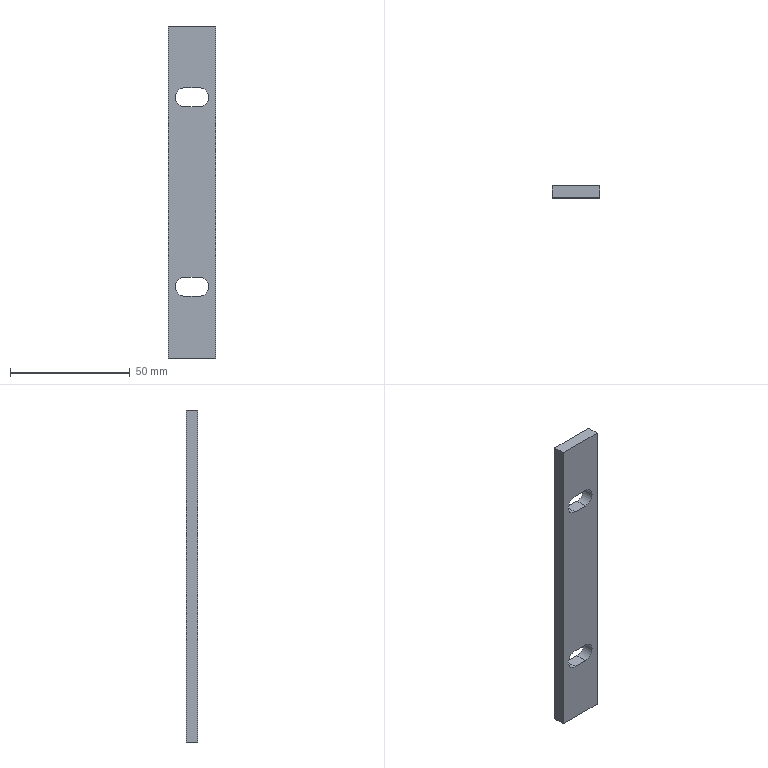Part | STEP file | PRT0001_68_17 | 1 solid | 14 faces | box 20 x 5 x 138.552 mm | volume 12873 mm3 | plane 10 | cylinder 4 | commonest cylinder face diameters 8 x4
STEP:
#1=CARTESIAN_POINT('',(0.,0.,0.));
#2=DIRECTION('',(0.,0.,1.));
#3=DIRECTION('',(1.,0.,0.));
#4=AXIS2_PLACEMENT_3D('',#1,#2,#3);
#5=CARTESIAN_POINT('',(1371.462,1237.457,35.5));
#6=VERTEX_POINT('',#5);
#7=CARTESIAN_POINT('',(1377.462,1237.457,35.5));
#8=VERTEX_POINT('',#7);
#9=CARTESIAN_POINT('',(1371.462,1237.457,35.5));
#10=DIRECTION('',(1.,0.,0.));
#11=VECTOR('',#10,1.);
#12=LINE('',#9,#11);
#13=CARTESIAN_POINT('',(1377.462,1242.457,35.5));
#14=DIRECTION('',(0.,0.,-1.));
#15=DIRECTION('',(-1.,0.,0.));
#16=AXIS2_PLACEMENT_3D('',#13,#14,#15);
#17=PLANE('',#16);
#18=CARTESIAN_POINT('',(6.,-5.));
#19=DIRECTION('',(-1.,0.));
#20=VECTOR('',#19,1.);
#21=LINE('',#18,#20);
#22=(GEOMETRIC_REPRESENTATION_CONTEXT(2)PARAMETRIC_REPRESENTATION_CONTEXT()REPRESENTATION_CONTEXT('',''));
#23=DEFINITIONAL_REPRESENTATION('',(#21),#22);
#24=PCURVE('',#17,#23);
#25=CARTESIAN_POINT('',(1364.462,1237.457,72.014));
#26=DIRECTION('',(0.,-1.,0.));
#27=DIRECTION('',(1.,0.,0.));
#28=AXIS2_PLACEMENT_3D('',#25,#26,#27);
#29=PLANE('',#28);
#30=CARTESIAN_POINT('',(7.,-36.514));
#31=DIRECTION('',(1.,0.));
#32=VECTOR('',#31,1.);
#33=LINE('',#30,#32);
#34=(GEOMETRIC_REPRESENTATION_CONTEXT(2)PARAMETRIC_REPRESENTATION_CONTEXT()REPRESENTATION_CONTEXT('',''));
#35=DEFINITIONAL_REPRESENTATION('',(#33),#34);
#36=PCURVE('',#29,#35);
#37=SURFACE_CURVE('',#12,(#24,#36),.PCURVE_S1.);
#38=EDGE_CURVE('',#6,#8,#37,.T.);
#39=ORIENTED_EDGE('',*,*,#38,.F.);
#40=CARTESIAN_POINT('',(1371.462,1242.457,35.5));
#41=VERTEX_POINT('',#40);
#42=CARTESIAN_POINT('',(1371.462,1242.457,35.5));
#43=DIRECTION('',(0.,-1.,0.));
#44=VECTOR('',#43,1.);
#45=LINE('',#42,#44);
#46=CARTESIAN_POINT('',(6.,0.00006163));
#47=DIRECTION('',(0.,-1.));
#48=VECTOR('',#47,1.);
#49=LINE('',#46,#48);
#50=(GEOMETRIC_REPRESENTATION_CONTEXT(2)PARAMETRIC_REPRESENTATION_CONTEXT()REPRESENTATION_CONTEXT('',''));
#51=DEFINITIONAL_REPRESENTATION('',(#49),#50);
#52=PCURVE('',#17,#51);
#53=CARTESIAN_POINT('',(1371.462,1242.457,39.5));
#54=DIRECTION('',(0.,1.,0.));
#55=DIRECTION('',(1.,0.,0.));
#56=AXIS2_PLACEMENT_3D('',#53,#54,#55);
#57=CYLINDRICAL_SURFACE('',#56,4.);
#58=CARTESIAN_POINT('',(1.571,0.00006163));
#59=DIRECTION('',(0.,-1.));
#60=VECTOR('',#59,1.);
#61=LINE('',#58,#60);
#62=(GEOMETRIC_REPRESENTATION_CONTEXT(2)PARAMETRIC_REPRESENTATION_CONTEXT()REPRESENTATION_CONTEXT('',''));
#63=DEFINITIONAL_REPRESENTATION('',(#61),#62);
#64=PCURVE('',#57,#63);
#65=SURFACE_CURVE('',#45,(#52,#64),.PCURVE_S1.);
#66=EDGE_CURVE('',#41,#6,#65,.T.);
#67=ORIENTED_EDGE('',*,*,#66,.F.);
#68=CARTESIAN_POINT('',(1377.462,1242.457,35.5));
#69=VERTEX_POINT('',#68);
#70=CARTESIAN_POINT('',(1371.462,1242.457,35.5));
#71=DIRECTION('',(1.,0.,0.));
#72=VECTOR('',#71,1.);
#73=LINE('',#70,#72);
#74=CARTESIAN_POINT('',(6.,0.00006163));
#75=DIRECTION('',(-1.,0.));
#76=VECTOR('',#75,1.);
#77=LINE('',#74,#76);
#78=(GEOMETRIC_REPRESENTATION_CONTEXT(2)PARAMETRIC_REPRESENTATION_CONTEXT()REPRESENTATION_CONTEXT('',''));
#79=DEFINITIONAL_REPRESENTATION('',(#77),#78);
#80=PCURVE('',#17,#79);
#81=CARTESIAN_POINT('',(1384.462,1242.457,72.014));
#82=DIRECTION('',(0.,1.,0.));
#83=DIRECTION('',(-1.,0.,0.));
#84=AXIS2_PLACEMENT_3D('',#81,#82,#83);
#85=PLANE('',#84);
#86=CARTESIAN_POINT('',(13.,-36.514));
#87=DIRECTION('',(-1.,0.));
#88=VECTOR('',#87,1.);
#89=LINE('',#86,#88);
#90=(GEOMETRIC_REPRESENTATION_CONTEXT(2)PARAMETRIC_REPRESENTATION_CONTEXT()REPRESENTATION_CONTEXT('',''));
#91=DEFINITIONAL_REPRESENTATION('',(#89),#90);
#92=PCURVE('',#85,#91);
#93=SURFACE_CURVE('',#73,(#80,#92),.PCURVE_S1.);
#94=EDGE_CURVE('',#41,#69,#93,.T.);
#95=ORIENTED_EDGE('',*,*,#94,.T.);
#96=CARTESIAN_POINT('',(1377.462,1237.457,35.5));
#97=DIRECTION('',(0.,1.,0.));
#98=VECTOR('',#97,1.);
#99=LINE('',#96,#98);
#100=CARTESIAN_POINT('',(0.,-5.));
#101=DIRECTION('',(0.,1.));
#102=VECTOR('',#101,1.);
#103=LINE('',#100,#102);
#104=(GEOMETRIC_REPRESENTATION_CONTEXT(2)PARAMETRIC_REPRESENTATION_CONTEXT()REPRESENTATION_CONTEXT('',''));
#105=DEFINITIONAL_REPRESENTATION('',(#103),#104);
#106=PCURVE('',#17,#105);
#107=CARTESIAN_POINT('',(1377.462,1242.457,39.5));
#108=DIRECTION('',(0.,1.,0.));
#109=DIRECTION('',(1.,0.,0.));
#110=AXIS2_PLACEMENT_3D('',#107,#108,#109);
#111=CYLINDRICAL_SURFACE('',#110,4.);
#112=CARTESIAN_POINT('',(1.571,-5.));
#113=DIRECTION('',(0.,1.));
#114=VECTOR('',#113,1.);
#115=LINE('',#112,#114);
#116=(GEOMETRIC_REPRESENTATION_CONTEXT(2)PARAMETRIC_REPRESENTATION_CONTEXT()REPRESENTATION_CONTEXT('',''));
#117=DEFINITIONAL_REPRESENTATION('',(#115),#116);
#118=PCURVE('',#111,#117);
#119=SURFACE_CURVE('',#99,(#106,#118),.PCURVE_S1.);
#120=EDGE_CURVE('',#8,#69,#119,.T.);
#121=ORIENTED_EDGE('',*,*,#120,.F.);
#122=EDGE_LOOP('',(#39,#67,#95,#121));
#123=FACE_BOUND('',#122,.F.);
#124=ADVANCED_FACE('',(#123),#17,.F.);
#125=CARTESIAN_POINT('',(1384.462,1237.457,-69.276));
#126=VERTEX_POINT('',#125);
#127=CARTESIAN_POINT('',(1364.462,1237.457,-69.276));
#128=VERTEX_POINT('',#127);
#129=CARTESIAN_POINT('',(1384.462,1237.457,-69.276));
#130=DIRECTION('',(-1.,0.,0.));
#131=VECTOR('',#130,1.);
#132=LINE('',#129,#131);
#133=CARTESIAN_POINT('',(20.,-141.29));
#134=DIRECTION('',(-1.,0.));
#135=VECTOR('',#134,1.);
#136=LINE('',#133,#135);
#137=(GEOMETRIC_REPRESENTATION_CONTEXT(2)PARAMETRIC_REPRESENTATION_CONTEXT()REPRESENTATION_CONTEXT('',''));
#138=DEFINITIONAL_REPRESENTATION('',(#136),#137);
#139=PCURVE('',#29,#138);
#140=CARTESIAN_POINT('',(1605.102,1107.827,-69.276));
#141=DIRECTION('',(0.,0.,-1.));
#142=DIRECTION('',(-1.,0.,0.));
#143=AXIS2_PLACEMENT_3D('',#140,#141,#142);
#144=PLANE('',#143);
#145=CARTESIAN_POINT('',(220.639,129.63));
#146=DIRECTION('',(1.,0.));
#147=VECTOR('',#146,1.);
#148=LINE('',#145,#147);
#149=(GEOMETRIC_REPRESENTATION_CONTEXT(2)PARAMETRIC_REPRESENTATION_CONTEXT()REPRESENTATION_CONTEXT('',''));
#150=DEFINITIONAL_REPRESENTATION('',(#148),#149);
#151=PCURVE('',#144,#150);
#152=SURFACE_CURVE('',#132,(#139,#151),.PCURVE_S1.);
#153=EDGE_CURVE('',#126,#128,#152,.T.);
#154=ORIENTED_EDGE('',*,*,#153,.T.);
#155=CARTESIAN_POINT('',(1364.462,1237.457,69.276));
#156=VERTEX_POINT('',#155);
#157=CARTESIAN_POINT('',(1364.462,1237.457,69.276));
#158=DIRECTION('',(0.,0.,-1.));
#159=VECTOR('',#158,1.);
#160=LINE('',#157,#159);
#161=CARTESIAN_POINT('',(0.,-2.738));
#162=DIRECTION('',(0.,-1.));
#163=VECTOR('',#162,1.);
#164=LINE('',#161,#163);
#165=(GEOMETRIC_REPRESENTATION_CONTEXT(2)PARAMETRIC_REPRESENTATION_CONTEXT()REPRESENTATION_CONTEXT('',''));
#166=DEFINITIONAL_REPRESENTATION('',(#164),#165);
#167=PCURVE('',#29,#166);
#168=CARTESIAN_POINT('',(1364.462,1242.457,72.014));
#169=DIRECTION('',(-1.,0.,0.));
#170=DIRECTION('',(0.,-1.,0.));
#171=AXIS2_PLACEMENT_3D('',#168,#169,#170);
#172=PLANE('',#171);
#173=CARTESIAN_POINT('',(5.,-2.738));
#174=DIRECTION('',(0.,-1.));
#175=VECTOR('',#174,1.);
#176=LINE('',#173,#175);
#177=(GEOMETRIC_REPRESENTATION_CONTEXT(2)PARAMETRIC_REPRESENTATION_CONTEXT()REPRESENTATION_CONTEXT('',''));
#178=DEFINITIONAL_REPRESENTATION('',(#176),#177);
#179=PCURVE('',#172,#178);
#180=SURFACE_CURVE('',#160,(#167,#179),.PCURVE_S1.);
#181=EDGE_CURVE('',#156,#128,#180,.T.);
#182=ORIENTED_EDGE('',*,*,#181,.F.);
#183=CARTESIAN_POINT('',(1384.462,1237.457,69.276));
#184=VERTEX_POINT('',#183);
#185=CARTESIAN_POINT('',(1384.462,1237.457,69.276));
#186=DIRECTION('',(-1.,0.,0.));
#187=VECTOR('',#186,1.);
#188=LINE('',#185,#187);
#189=CARTESIAN_POINT('',(20.,-2.738));
#190=DIRECTION('',(-1.,0.));
#191=VECTOR('',#190,1.);
#192=LINE('',#189,#191);
#193=(GEOMETRIC_REPRESENTATION_CONTEXT(2)PARAMETRIC_REPRESENTATION_CONTEXT()REPRESENTATION_CONTEXT('',''));
#194=DEFINITIONAL_REPRESENTATION('',(#192),#193);
#195=PCURVE('',#29,#194);
#196=CARTESIAN_POINT('',(1356.569,1107.827,69.276));
#197=DIRECTION('',(0.,0.,1.));
#198=DIRECTION('',(1.,0.,0.));
#199=AXIS2_PLACEMENT_3D('',#196,#197,#198);
#200=PLANE('',#199);
#201=CARTESIAN_POINT('',(27.893,129.63));
#202=DIRECTION('',(-1.,0.));
#203=VECTOR('',#202,1.);
#204=LINE('',#201,#203);
#205=(GEOMETRIC_REPRESENTATION_CONTEXT(2)PARAMETRIC_REPRESENTATION_CONTEXT()REPRESENTATION_CONTEXT('',''));
#206=DEFINITIONAL_REPRESENTATION('',(#204),#205);
#207=PCURVE('',#200,#206);
#208=SURFACE_CURVE('',#188,(#195,#207),.PCURVE_S1.);
#209=EDGE_CURVE('',#184,#156,#208,.T.);
#210=ORIENTED_EDGE('',*,*,#209,.F.);
#211=CARTESIAN_POINT('',(1384.462,1237.457,69.276));
#212=DIRECTION('',(0.,0.,-1.));
#213=VECTOR('',#212,1.);
#214=LINE('',#211,#213);
#215=CARTESIAN_POINT('',(20.,-2.738));
#216=DIRECTION('',(0.,-1.));
#217=VECTOR('',#216,1.);
#218=LINE('',#215,#217);
#219=(GEOMETRIC_REPRESENTATION_CONTEXT(2)PARAMETRIC_REPRESENTATION_CONTEXT()REPRESENTATION_CONTEXT('',''));
#220=DEFINITIONAL_REPRESENTATION('',(#218),#219);
#221=PCURVE('',#29,#220);
#222=CARTESIAN_POINT('',(1384.462,1237.457,72.014));
#223=DIRECTION('',(1.,0.,0.));
#224=DIRECTION('',(0.,1.,0.));
#225=AXIS2_PLACEMENT_3D('',#222,#223,#224);
#226=PLANE('',#225);
#227=CARTESIAN_POINT('',(0.,-2.738));
#228=DIRECTION('',(0.,-1.));
#229=VECTOR('',#228,1.);
#230=LINE('',#227,#229);
#231=(GEOMETRIC_REPRESENTATION_CONTEXT(2)PARAMETRIC_REPRESENTATION_CONTEXT()REPRESENTATION_CONTEXT('',''));
#232=DEFINITIONAL_REPRESENTATION('',(#230),#231);
#233=PCURVE('',#226,#232);
#234=SURFACE_CURVE('',#214,(#221,#233),.PCURVE_S1.);
#235=EDGE_CURVE('',#184,#126,#234,.T.);
#236=ORIENTED_EDGE('',*,*,#235,.T.);
#237=EDGE_LOOP('',(#154,#182,#210,#236));
#238=FACE_BOUND('',#237,.F.);
#239=CARTESIAN_POINT('',(1377.462,1237.457,-35.5));
#240=VERTEX_POINT('',#239);
#241=CARTESIAN_POINT('',(1371.462,1237.457,-35.5));
#242=VERTEX_POINT('',#241);
#243=CARTESIAN_POINT('',(1377.462,1237.457,-35.5));
#244=DIRECTION('',(-1.,0.,0.));
#245=VECTOR('',#244,1.);
#246=LINE('',#243,#245);
#247=CARTESIAN_POINT('',(13.,-107.514));
#248=DIRECTION('',(-1.,0.));
#249=VECTOR('',#248,1.);
#250=LINE('',#247,#249);
#251=(GEOMETRIC_REPRESENTATION_CONTEXT(2)PARAMETRIC_REPRESENTATION_CONTEXT()REPRESENTATION_CONTEXT('',''));
#252=DEFINITIONAL_REPRESENTATION('',(#250),#251);
#253=PCURVE('',#29,#252);
#254=CARTESIAN_POINT('',(1371.462,1242.457,-35.5));
#255=DIRECTION('',(0.,0.,1.));
#256=DIRECTION('',(1.,0.,0.));
#257=AXIS2_PLACEMENT_3D('',#254,#255,#256);
#258=PLANE('',#257);
#259=CARTESIAN_POINT('',(6.,-5.));
#260=DIRECTION('',(-1.,0.));
#261=VECTOR('',#260,1.);
#262=LINE('',#259,#261);
#263=(GEOMETRIC_REPRESENTATION_CONTEXT(2)PARAMETRIC_REPRESENTATION_CONTEXT()REPRESENTATION_CONTEXT('',''));
#264=DEFINITIONAL_REPRESENTATION('',(#262),#263);
#265=PCURVE('',#258,#264);
#266=SURFACE_CURVE('',#246,(#253,#265),.PCURVE_S1.);
#267=EDGE_CURVE('',#240,#242,#266,.T.);
#268=ORIENTED_EDGE('',*,*,#267,.T.);
#269=CARTESIAN_POINT('',(1367.462,1237.457,-39.5));
#270=VERTEX_POINT('',#269);
#271=CARTESIAN_POINT('',(1371.462,1237.457,-39.5));
#272=DIRECTION('',(0.,-1.,0.));
#273=DIRECTION('',(0.,0.,1.));
#274=AXIS2_PLACEMENT_3D('',#271,#272,#273);
#275=CIRCLE('',#274,4.);
#276=CARTESIAN_POINT('',(7.,-111.514));
#277=DIRECTION('',(0.,1.));
#278=AXIS2_PLACEMENT_2D('',#276,#277);
#279=CIRCLE('',#278,4.);
#280=(GEOMETRIC_REPRESENTATION_CONTEXT(2)PARAMETRIC_REPRESENTATION_CONTEXT()REPRESENTATION_CONTEXT('',''));
#281=DEFINITIONAL_REPRESENTATION('',(#279),#280);
#282=PCURVE('',#29,#281);
#283=CARTESIAN_POINT('',(1371.462,1242.457,-39.5));
#284=DIRECTION('',(0.,1.,0.));
#285=DIRECTION('',(1.,0.,0.));
#286=AXIS2_PLACEMENT_3D('',#283,#284,#285);
#287=CYLINDRICAL_SURFACE('',#286,4.);
#288=CARTESIAN_POINT('',(4.712,-5.));
#289=DIRECTION('',(-1.,0.));
#290=VECTOR('',#289,1.);
#291=LINE('',#288,#290);
#292=(GEOMETRIC_REPRESENTATION_CONTEXT(2)PARAMETRIC_REPRESENTATION_CONTEXT()REPRESENTATION_CONTEXT('',''));
#293=DEFINITIONAL_REPRESENTATION('',(#291),#292);
#294=PCURVE('',#287,#293);
#295=SURFACE_CURVE('',#275,(#282,#294),.PCURVE_S1.);
#296=EDGE_CURVE('',#242,#270,#295,.T.);
#297=ORIENTED_EDGE('',*,*,#296,.T.);
#298=CARTESIAN_POINT('',(1371.462,1237.457,-43.5));
#299=VERTEX_POINT('',#298);
#300=CARTESIAN_POINT('',(1371.462,1237.457,-39.5));
#301=DIRECTION('',(0.,-1.,0.));
#302=DIRECTION('',(-1.,0.,0.));
#303=AXIS2_PLACEMENT_3D('',#300,#301,#302);
#304=CIRCLE('',#303,4.);
#305=CARTESIAN_POINT('',(7.,-111.514));
#306=DIRECTION('',(-1.,0.));
#307=AXIS2_PLACEMENT_2D('',#305,#306);
#308=CIRCLE('',#307,4.);
#309=(GEOMETRIC_REPRESENTATION_CONTEXT(2)PARAMETRIC_REPRESENTATION_CONTEXT()REPRESENTATION_CONTEXT('',''));
#310=DEFINITIONAL_REPRESENTATION('',(#308),#309);
#311=PCURVE('',#29,#310);
#312=CARTESIAN_POINT('',(3.142,-5.));
#313=DIRECTION('',(-1.,0.));
#314=VECTOR('',#313,1.);
#315=LINE('',#312,#314);
#316=(GEOMETRIC_REPRESENTATION_CONTEXT(2)PARAMETRIC_REPRESENTATION_CONTEXT()REPRESENTATION_CONTEXT('',''));
#317=DEFINITIONAL_REPRESENTATION('',(#315),#316);
#318=PCURVE('',#287,#317);
#319=SURFACE_CURVE('',#304,(#311,#318),.PCURVE_S1.);
#320=EDGE_CURVE('',#270,#299,#319,.T.);
#321=ORIENTED_EDGE('',*,*,#320,.T.);
#322=CARTESIAN_POINT('',(1377.462,1237.457,-43.5));
#323=VERTEX_POINT('',#322);
#324=CARTESIAN_POINT('',(1371.462,1237.457,-43.5));
#325=DIRECTION('',(1.,0.,0.));
#326=VECTOR('',#325,1.);
#327=LINE('',#324,#326);
#328=CARTESIAN_POINT('',(7.,-115.514));
#329=DIRECTION('',(1.,0.));
#330=VECTOR('',#329,1.);
#331=LINE('',#328,#330);
#332=(GEOMETRIC_REPRESENTATION_CONTEXT(2)PARAMETRIC_REPRESENTATION_CONTEXT()REPRESENTATION_CONTEXT('',''));
#333=DEFINITIONAL_REPRESENTATION('',(#331),#332);
#334=PCURVE('',#29,#333);
#335=CARTESIAN_POINT('',(1377.462,1242.457,-43.5));
#336=DIRECTION('',(0.,0.,-1.));
#337=DIRECTION('',(-1.,0.,0.));
#338=AXIS2_PLACEMENT_3D('',#335,#336,#337);
#339=PLANE('',#338);
#340=CARTESIAN_POINT('',(6.,-5.));
#341=DIRECTION('',(-1.,0.));
#342=VECTOR('',#341,1.);
#343=LINE('',#340,#342);
#344=(GEOMETRIC_REPRESENTATION_CONTEXT(2)PARAMETRIC_REPRESENTATION_CONTEXT()REPRESENTATION_CONTEXT('',''));
#345=DEFINITIONAL_REPRESENTATION('',(#343),#344);
#346=PCURVE('',#339,#345);
#347=SURFACE_CURVE('',#327,(#334,#346),.PCURVE_S1.);
#348=EDGE_CURVE('',#299,#323,#347,.T.);
#349=ORIENTED_EDGE('',*,*,#348,.T.);
#350=CARTESIAN_POINT('',(1381.462,1237.457,-39.5));
#351=VERTEX_POINT('',#350);
#352=CARTESIAN_POINT('',(1377.462,1237.457,-39.5));
#353=DIRECTION('',(0.,-1.,0.));
#354=DIRECTION('',(0.,0.,-1.));
#355=AXIS2_PLACEMENT_3D('',#352,#353,#354);
#356=CIRCLE('',#355,4.);
#357=CARTESIAN_POINT('',(13.,-111.514));
#358=DIRECTION('',(0.,-1.));
#359=AXIS2_PLACEMENT_2D('',#357,#358);
#360=CIRCLE('',#359,4.);
#361=(GEOMETRIC_REPRESENTATION_CONTEXT(2)PARAMETRIC_REPRESENTATION_CONTEXT()REPRESENTATION_CONTEXT('',''));
#362=DEFINITIONAL_REPRESENTATION('',(#360),#361);
#363=PCURVE('',#29,#362);
#364=CARTESIAN_POINT('',(1377.462,1242.457,-39.5));
#365=DIRECTION('',(0.,1.,0.));
#366=DIRECTION('',(1.,0.,0.));
#367=AXIS2_PLACEMENT_3D('',#364,#365,#366);
#368=CYLINDRICAL_SURFACE('',#367,4.);
#369=CARTESIAN_POINT('',(1.571,-5.));
#370=DIRECTION('',(-1.,0.));
#371=VECTOR('',#370,1.);
#372=LINE('',#369,#371);
#373=(GEOMETRIC_REPRESENTATION_CONTEXT(2)PARAMETRIC_REPRESENTATION_CONTEXT()REPRESENTATION_CONTEXT('',''));
#374=DEFINITIONAL_REPRESENTATION('',(#372),#373);
#375=PCURVE('',#368,#374);
#376=SURFACE_CURVE('',#356,(#363,#375),.PCURVE_S1.);
#377=EDGE_CURVE('',#323,#351,#376,.T.);
#378=ORIENTED_EDGE('',*,*,#377,.T.);
#379=CARTESIAN_POINT('',(1377.462,1237.457,-39.5));
#380=DIRECTION('',(0.,-1.,0.));
#381=DIRECTION('',(1.,0.,0.));
#382=AXIS2_PLACEMENT_3D('',#379,#380,#381);
#383=CIRCLE('',#382,4.);
#384=CARTESIAN_POINT('',(13.,-111.514));
#385=DIRECTION('',(1.,0.));
#386=AXIS2_PLACEMENT_2D('',#384,#385);
#387=CIRCLE('',#386,4.);
#388=(GEOMETRIC_REPRESENTATION_CONTEXT(2)PARAMETRIC_REPRESENTATION_CONTEXT()REPRESENTATION_CONTEXT('',''));
#389=DEFINITIONAL_REPRESENTATION('',(#387),#388);
#390=PCURVE('',#29,#389);
#391=CARTESIAN_POINT('',(0.,-5.));
#392=DIRECTION('',(-1.,0.));
#393=VECTOR('',#392,1.);
#394=LINE('',#391,#393);
#395=(GEOMETRIC_REPRESENTATION_CONTEXT(2)PARAMETRIC_REPRESENTATION_CONTEXT()REPRESENTATION_CONTEXT('',''));
#396=DEFINITIONAL_REPRESENTATION('',(#394),#395);
#397=PCURVE('',#368,#396);
#398=SURFACE_CURVE('',#383,(#390,#397),.PCURVE_S1.);
#399=EDGE_CURVE('',#351,#240,#398,.T.);
#400=ORIENTED_EDGE('',*,*,#399,.T.);
#401=EDGE_LOOP('',(#268,#297,#321,#349,#378,#400));
#402=FACE_BOUND('',#401,.F.);
#403=CARTESIAN_POINT('',(1371.462,1237.457,43.5));
#404=VERTEX_POINT('',#403);
#405=CARTESIAN_POINT('',(1367.462,1237.457,39.5));
#406=VERTEX_POINT('',#405);
#407=CARTESIAN_POINT('',(1371.462,1237.457,39.5));
#408=DIRECTION('',(0.,-1.,0.));
#409=DIRECTION('',(0.,0.,1.));
#410=AXIS2_PLACEMENT_3D('',#407,#408,#409);
#411=CIRCLE('',#410,4.);
#412=CARTESIAN_POINT('',(7.,-32.514));
#413=DIRECTION('',(0.,1.));
#414=AXIS2_PLACEMENT_2D('',#412,#413);
#415=CIRCLE('',#414,4.);
#416=(GEOMETRIC_REPRESENTATION_CONTEXT(2)PARAMETRIC_REPRESENTATION_CONTEXT()REPRESENTATION_CONTEXT('',''));
#417=DEFINITIONAL_REPRESENTATION('',(#415),#416);
#418=PCURVE('',#29,#417);
#419=CARTESIAN_POINT('',(4.712,-5.));
#420=DIRECTION('',(-1.,0.));
#421=VECTOR('',#420,1.);
#422=LINE('',#419,#421);
#423=(GEOMETRIC_REPRESENTATION_CONTEXT(2)PARAMETRIC_REPRESENTATION_CONTEXT()REPRESENTATION_CONTEXT('',''));
#424=DEFINITIONAL_REPRESENTATION('',(#422),#423);
#425=PCURVE('',#57,#424);
#426=SURFACE_CURVE('',#411,(#418,#425),.PCURVE_S1.);
#427=EDGE_CURVE('',#404,#406,#426,.T.);
#428=ORIENTED_EDGE('',*,*,#427,.T.);
#429=CARTESIAN_POINT('',(1371.462,1237.457,39.5));
#430=DIRECTION('',(0.,-1.,0.));
#431=DIRECTION('',(-1.,0.,0.));
#432=AXIS2_PLACEMENT_3D('',#429,#430,#431);
#433=CIRCLE('',#432,4.);
#434=CARTESIAN_POINT('',(7.,-32.514));
#435=DIRECTION('',(-1.,0.));
#436=AXIS2_PLACEMENT_2D('',#434,#435);
#437=CIRCLE('',#436,4.);
#438=(GEOMETRIC_REPRESENTATION_CONTEXT(2)PARAMETRIC_REPRESENTATION_CONTEXT()REPRESENTATION_CONTEXT('',''));
#439=DEFINITIONAL_REPRESENTATION('',(#437),#438);
#440=PCURVE('',#29,#439);
#441=CARTESIAN_POINT('',(3.142,-5.));
#442=DIRECTION('',(-1.,0.));
#443=VECTOR('',#442,1.);
#444=LINE('',#441,#443);
#445=(GEOMETRIC_REPRESENTATION_CONTEXT(2)PARAMETRIC_REPRESENTATION_CONTEXT()REPRESENTATION_CONTEXT('',''));
#446=DEFINITIONAL_REPRESENTATION('',(#444),#445);
#447=PCURVE('',#57,#446);
#448=SURFACE_CURVE('',#433,(#440,#447),.PCURVE_S1.);
#449=EDGE_CURVE('',#406,#6,#448,.T.);
#450=ORIENTED_EDGE('',*,*,#449,.T.);
#451=ORIENTED_EDGE('',*,*,#38,.T.);
#452=CARTESIAN_POINT('',(1381.462,1237.457,39.5));
#453=VERTEX_POINT('',#452);
#454=CARTESIAN_POINT('',(1377.462,1237.457,39.5));
#455=DIRECTION('',(0.,-1.,0.));
#456=DIRECTION('',(0.,0.,-1.));
#457=AXIS2_PLACEMENT_3D('',#454,#455,#456);
#458=CIRCLE('',#457,4.);
#459=CARTESIAN_POINT('',(13.,-32.514));
#460=DIRECTION('',(0.,-1.));
#461=AXIS2_PLACEMENT_2D('',#459,#460);
#462=CIRCLE('',#461,4.);
#463=(GEOMETRIC_REPRESENTATION_CONTEXT(2)PARAMETRIC_REPRESENTATION_CONTEXT()REPRESENTATION_CONTEXT('',''));
#464=DEFINITIONAL_REPRESENTATION('',(#462),#463);
#465=PCURVE('',#29,#464);
#466=CARTESIAN_POINT('',(1.571,-5.));
#467=DIRECTION('',(-1.,0.));
#468=VECTOR('',#467,1.);
#469=LINE('',#466,#468);
#470=(GEOMETRIC_REPRESENTATION_CONTEXT(2)PARAMETRIC_REPRESENTATION_CONTEXT()REPRESENTATION_CONTEXT('',''));
#471=DEFINITIONAL_REPRESENTATION('',(#469),#470);
#472=PCURVE('',#111,#471);
#473=SURFACE_CURVE('',#458,(#465,#472),.PCURVE_S1.);
#474=EDGE_CURVE('',#8,#453,#473,.T.);
#475=ORIENTED_EDGE('',*,*,#474,.T.);
#476=CARTESIAN_POINT('',(1377.462,1237.457,43.5));
#477=VERTEX_POINT('',#476);
#478=CARTESIAN_POINT('',(1377.462,1237.457,39.5));
#479=DIRECTION('',(0.,-1.,0.));
#480=DIRECTION('',(1.,0.,0.));
#481=AXIS2_PLACEMENT_3D('',#478,#479,#480);
#482=CIRCLE('',#481,4.);
#483=CARTESIAN_POINT('',(13.,-32.514));
#484=DIRECTION('',(1.,0.));
#485=AXIS2_PLACEMENT_2D('',#483,#484);
#486=CIRCLE('',#485,4.);
#487=(GEOMETRIC_REPRESENTATION_CONTEXT(2)PARAMETRIC_REPRESENTATION_CONTEXT()REPRESENTATION_CONTEXT('',''));
#488=DEFINITIONAL_REPRESENTATION('',(#486),#487);
#489=PCURVE('',#29,#488);
#490=CARTESIAN_POINT('',(0.,-5.));
#491=DIRECTION('',(-1.,0.));
#492=VECTOR('',#491,1.);
#493=LINE('',#490,#492);
#494=(GEOMETRIC_REPRESENTATION_CONTEXT(2)PARAMETRIC_REPRESENTATION_CONTEXT()REPRESENTATION_CONTEXT('',''));
#495=DEFINITIONAL_REPRESENTATION('',(#493),#494);
#496=PCURVE('',#111,#495);
#497=SURFACE_CURVE('',#482,(#489,#496),.PCURVE_S1.);
#498=EDGE_CURVE('',#453,#477,#497,.T.);
#499=ORIENTED_EDGE('',*,*,#498,.T.);
#500=CARTESIAN_POINT('',(1377.462,1237.457,43.5));
#501=DIRECTION('',(-1.,0.,0.));
#502=VECTOR('',#501,1.);
#503=LINE('',#500,#502);
#504=CARTESIAN_POINT('',(13.,-28.514));
#505=DIRECTION('',(-1.,0.));
#506=VECTOR('',#505,1.);
#507=LINE('',#504,#506);
#508=(GEOMETRIC_REPRESENTATION_CONTEXT(2)PARAMETRIC_REPRESENTATION_CONTEXT()REPRESENTATION_CONTEXT('',''));
#509=DEFINITIONAL_REPRESENTATION('',(#507),#508);
#510=PCURVE('',#29,#509);
#511=CARTESIAN_POINT('',(1371.462,1242.457,43.5));
#512=DIRECTION('',(0.,0.,1.));
#513=DIRECTION('',(1.,0.,0.));
#514=AXIS2_PLACEMENT_3D('',#511,#512,#513);
#515=PLANE('',#514);
#516=CARTESIAN_POINT('',(6.,-5.));
#517=DIRECTION('',(-1.,0.));
#518=VECTOR('',#517,1.);
#519=LINE('',#516,#518);
#520=(GEOMETRIC_REPRESENTATION_CONTEXT(2)PARAMETRIC_REPRESENTATION_CONTEXT()REPRESENTATION_CONTEXT('',''));
#521=DEFINITIONAL_REPRESENTATION('',(#519),#520);
#522=PCURVE('',#515,#521);
#523=SURFACE_CURVE('',#503,(#510,#522),.PCURVE_S1.);
#524=EDGE_CURVE('',#477,#404,#523,.T.);
#525=ORIENTED_EDGE('',*,*,#524,.T.);
#526=EDGE_LOOP('',(#428,#450,#451,#475,#499,#525));
#527=FACE_BOUND('',#526,.F.);
#528=ADVANCED_FACE('',(#238,#402,#527),#29,.T.);
#529=CARTESIAN_POINT('',(1364.462,1242.457,-69.276));
#530=VERTEX_POINT('',#529);
#531=CARTESIAN_POINT('',(1364.462,1237.457,-69.276));
#532=DIRECTION('',(0.,1.,0.));
#533=VECTOR('',#532,1.);
#534=LINE('',#531,#533);
#535=CARTESIAN_POINT('',(240.639,129.63));
#536=DIRECTION('',(0.,1.));
#537=VECTOR('',#536,1.);
#538=LINE('',#535,#537);
#539=(GEOMETRIC_REPRESENTATION_CONTEXT(2)PARAMETRIC_REPRESENTATION_CONTEXT()REPRESENTATION_CONTEXT('',''));
#540=DEFINITIONAL_REPRESENTATION('',(#538),#539);
#541=PCURVE('',#144,#540);
#542=CARTESIAN_POINT('',(5.,-141.29));
#543=DIRECTION('',(-1.,0.));
#544=VECTOR('',#543,1.);
#545=LINE('',#542,#544);
#546=(GEOMETRIC_REPRESENTATION_CONTEXT(2)PARAMETRIC_REPRESENTATION_CONTEXT()REPRESENTATION_CONTEXT('',''));
#547=DEFINITIONAL_REPRESENTATION('',(#545),#546);
#548=PCURVE('',#172,#547);
#549=SURFACE_CURVE('',#534,(#541,#548),.PCURVE_S1.);
#550=EDGE_CURVE('',#128,#530,#549,.T.);
#551=ORIENTED_EDGE('',*,*,#550,.F.);
#552=ORIENTED_EDGE('',*,*,#153,.F.);
#553=CARTESIAN_POINT('',(1384.462,1242.457,-69.276));
#554=VERTEX_POINT('',#553);
#555=CARTESIAN_POINT('',(1384.462,1242.457,-69.276));
#556=DIRECTION('',(0.,-1.,0.));
#557=VECTOR('',#556,1.);
#558=LINE('',#555,#557);
#559=CARTESIAN_POINT('',(220.639,134.63));
#560=DIRECTION('',(0.,-1.));
#561=VECTOR('',#560,1.);
#562=LINE('',#559,#561);
#563=(GEOMETRIC_REPRESENTATION_CONTEXT(2)PARAMETRIC_REPRESENTATION_CONTEXT()REPRESENTATION_CONTEXT('',''));
#564=DEFINITIONAL_REPRESENTATION('',(#562),#563);
#565=PCURVE('',#144,#564);
#566=CARTESIAN_POINT('',(5.,-141.29));
#567=DIRECTION('',(-1.,0.));
#568=VECTOR('',#567,1.);
#569=LINE('',#566,#568);
#570=(GEOMETRIC_REPRESENTATION_CONTEXT(2)PARAMETRIC_REPRESENTATION_CONTEXT()REPRESENTATION_CONTEXT('',''));
#571=DEFINITIONAL_REPRESENTATION('',(#569),#570);
#572=PCURVE('',#226,#571);
#573=SURFACE_CURVE('',#558,(#565,#572),.PCURVE_S1.);
#574=EDGE_CURVE('',#554,#126,#573,.T.);
#575=ORIENTED_EDGE('',*,*,#574,.F.);
#576=CARTESIAN_POINT('',(1364.462,1242.457,-69.276));
#577=DIRECTION('',(1.,0.,0.));
#578=VECTOR('',#577,1.);
#579=LINE('',#576,#578);
#580=CARTESIAN_POINT('',(240.639,134.63));
#581=DIRECTION('',(-1.,0.));
#582=VECTOR('',#581,1.);
#583=LINE('',#580,#582);
#584=(GEOMETRIC_REPRESENTATION_CONTEXT(2)PARAMETRIC_REPRESENTATION_CONTEXT()REPRESENTATION_CONTEXT('',''));
#585=DEFINITIONAL_REPRESENTATION('',(#583),#584);
#586=PCURVE('',#144,#585);
#587=CARTESIAN_POINT('',(20.,-141.29));
#588=DIRECTION('',(-1.,0.));
#589=VECTOR('',#588,1.);
#590=LINE('',#587,#589);
#591=(GEOMETRIC_REPRESENTATION_CONTEXT(2)PARAMETRIC_REPRESENTATION_CONTEXT()REPRESENTATION_CONTEXT('',''));
#592=DEFINITIONAL_REPRESENTATION('',(#590),#591);
#593=PCURVE('',#85,#592);
#594=SURFACE_CURVE('',#579,(#586,#593),.PCURVE_S1.);
#595=EDGE_CURVE('',#530,#554,#594,.T.);
#596=ORIENTED_EDGE('',*,*,#595,.F.);
#597=EDGE_LOOP('',(#551,#552,#575,#596));
#598=FACE_BOUND('',#597,.F.);
#599=ADVANCED_FACE('',(#598),#144,.T.);
#600=ORIENTED_EDGE('',*,*,#550,.T.);
#601=CARTESIAN_POINT('',(1364.462,1242.457,69.276));
#602=VERTEX_POINT('',#601);
#603=CARTESIAN_POINT('',(1364.462,1242.457,69.276));
#604=DIRECTION('',(0.,0.,-1.));
#605=VECTOR('',#604,1.);
#606=LINE('',#603,#605);
#607=CARTESIAN_POINT('',(0.,-2.738));
#608=DIRECTION('',(0.,-1.));
#609=VECTOR('',#608,1.);
#610=LINE('',#607,#609);
#611=(GEOMETRIC_REPRESENTATION_CONTEXT(2)PARAMETRIC_REPRESENTATION_CONTEXT()REPRESENTATION_CONTEXT('',''));
#612=DEFINITIONAL_REPRESENTATION('',(#610),#611);
#613=PCURVE('',#172,#612);
#614=CARTESIAN_POINT('',(20.,-2.738));
#615=DIRECTION('',(0.,-1.));
#616=VECTOR('',#615,1.);
#617=LINE('',#614,#616);
#618=(GEOMETRIC_REPRESENTATION_CONTEXT(2)PARAMETRIC_REPRESENTATION_CONTEXT()REPRESENTATION_CONTEXT('',''));
#619=DEFINITIONAL_REPRESENTATION('',(#617),#618);
#620=PCURVE('',#85,#619);
#621=SURFACE_CURVE('',#606,(#613,#620),.PCURVE_S1.);
#622=EDGE_CURVE('',#602,#530,#621,.T.);
#623=ORIENTED_EDGE('',*,*,#622,.F.);
#624=CARTESIAN_POINT('',(1364.462,1237.457,69.276));
#625=DIRECTION('',(0.,1.,0.));
#626=VECTOR('',#625,1.);
#627=LINE('',#624,#626);
#628=CARTESIAN_POINT('',(5.,-2.738));
#629=DIRECTION('',(-1.,0.));
#630=VECTOR('',#629,1.);
#631=LINE('',#628,#630);
#632=(GEOMETRIC_REPRESENTATION_CONTEXT(2)PARAMETRIC_REPRESENTATION_CONTEXT()REPRESENTATION_CONTEXT('',''));
#633=DEFINITIONAL_REPRESENTATION('',(#631),#632);
#634=PCURVE('',#172,#633);
#635=CARTESIAN_POINT('',(7.893,129.63));
#636=DIRECTION('',(0.,1.));
#637=VECTOR('',#636,1.);
#638=LINE('',#635,#637);
#639=(GEOMETRIC_REPRESENTATION_CONTEXT(2)PARAMETRIC_REPRESENTATION_CONTEXT()REPRESENTATION_CONTEXT('',''));
#640=DEFINITIONAL_REPRESENTATION('',(#638),#639);
#641=PCURVE('',#200,#640);
#642=SURFACE_CURVE('',#627,(#634,#641),.PCURVE_S1.);
#643=EDGE_CURVE('',#156,#602,#642,.T.);
#644=ORIENTED_EDGE('',*,*,#643,.F.);
#645=ORIENTED_EDGE('',*,*,#181,.T.);
#646=EDGE_LOOP('',(#600,#623,#644,#645));
#647=FACE_BOUND('',#646,.F.);
#648=ADVANCED_FACE('',(#647),#172,.T.);
#649=ORIENTED_EDGE('',*,*,#595,.T.);
#650=CARTESIAN_POINT('',(1384.462,1242.457,69.276));
#651=VERTEX_POINT('',#650);
#652=CARTESIAN_POINT('',(1384.462,1242.457,69.276));
#653=DIRECTION('',(0.,0.,-1.));
#654=VECTOR('',#653,1.);
#655=LINE('',#652,#654);
#656=CARTESIAN_POINT('',(0.,-2.738));
#657=DIRECTION('',(0.,-1.));
#658=VECTOR('',#657,1.);
#659=LINE('',#656,#658);
#660=(GEOMETRIC_REPRESENTATION_CONTEXT(2)PARAMETRIC_REPRESENTATION_CONTEXT()REPRESENTATION_CONTEXT('',''));
#661=DEFINITIONAL_REPRESENTATION('',(#659),#660);
#662=PCURVE('',#85,#661);
#663=CARTESIAN_POINT('',(5.,-2.738));
#664=DIRECTION('',(0.,-1.));
#665=VECTOR('',#664,1.);
#666=LINE('',#663,#665);
#667=(GEOMETRIC_REPRESENTATION_CONTEXT(2)PARAMETRIC_REPRESENTATION_CONTEXT()REPRESENTATION_CONTEXT('',''));
#668=DEFINITIONAL_REPRESENTATION('',(#666),#667);
#669=PCURVE('',#226,#668);
#670=SURFACE_CURVE('',#655,(#662,#669),.PCURVE_S1.);
#671=EDGE_CURVE('',#651,#554,#670,.T.);
#672=ORIENTED_EDGE('',*,*,#671,.F.);
#673=CARTESIAN_POINT('',(1364.462,1242.457,69.276));
#674=DIRECTION('',(1.,0.,0.));
#675=VECTOR('',#674,1.);
#676=LINE('',#673,#675);
#677=CARTESIAN_POINT('',(20.,-2.738));
#678=DIRECTION('',(-1.,0.));
#679=VECTOR('',#678,1.);
#680=LINE('',#677,#679);
#681=(GEOMETRIC_REPRESENTATION_CONTEXT(2)PARAMETRIC_REPRESENTATION_CONTEXT()REPRESENTATION_CONTEXT('',''));
#682=DEFINITIONAL_REPRESENTATION('',(#680),#681);
#683=PCURVE('',#85,#682);
#684=CARTESIAN_POINT('',(7.893,134.63));
#685=DIRECTION('',(1.,0.));
#686=VECTOR('',#685,1.);
#687=LINE('',#684,#686);
#688=(GEOMETRIC_REPRESENTATION_CONTEXT(2)PARAMETRIC_REPRESENTATION_CONTEXT()REPRESENTATION_CONTEXT('',''));
#689=DEFINITIONAL_REPRESENTATION('',(#687),#688);
#690=PCURVE('',#200,#689);
#691=SURFACE_CURVE('',#676,(#683,#690),.PCURVE_S1.);
#692=EDGE_CURVE('',#602,#651,#691,.T.);
#693=ORIENTED_EDGE('',*,*,#692,.F.);
#694=ORIENTED_EDGE('',*,*,#622,.T.);
#695=EDGE_LOOP('',(#649,#672,#693,#694));
#696=FACE_BOUND('',#695,.F.);
#697=CARTESIAN_POINT('',(1377.462,1242.457,-35.5));
#698=VERTEX_POINT('',#697);
#699=CARTESIAN_POINT('',(1371.462,1242.457,-35.5));
#700=VERTEX_POINT('',#699);
#701=CARTESIAN_POINT('',(1377.462,1242.457,-35.5));
#702=DIRECTION('',(-1.,0.,0.));
#703=VECTOR('',#702,1.);
#704=LINE('',#701,#703);
#705=CARTESIAN_POINT('',(7.,-107.514));
#706=DIRECTION('',(1.,0.));
#707=VECTOR('',#706,1.);
#708=LINE('',#705,#707);
#709=(GEOMETRIC_REPRESENTATION_CONTEXT(2)PARAMETRIC_REPRESENTATION_CONTEXT()REPRESENTATION_CONTEXT('',''));
#710=DEFINITIONAL_REPRESENTATION('',(#708),#709);
#711=PCURVE('',#85,#710);
#712=CARTESIAN_POINT('',(6.,0.00006163));
#713=DIRECTION('',(-1.,0.));
#714=VECTOR('',#713,1.);
#715=LINE('',#712,#714);
#716=(GEOMETRIC_REPRESENTATION_CONTEXT(2)PARAMETRIC_REPRESENTATION_CONTEXT()REPRESENTATION_CONTEXT('',''));
#717=DEFINITIONAL_REPRESENTATION('',(#715),#716);
#718=PCURVE('',#258,#717);
#719=SURFACE_CURVE('',#704,(#711,#718),.PCURVE_S1.);
#720=EDGE_CURVE('',#698,#700,#719,.T.);
#721=ORIENTED_EDGE('',*,*,#720,.F.);
#722=CARTESIAN_POINT('',(1381.462,1242.457,-39.5));
#723=VERTEX_POINT('',#722);
#724=CARTESIAN_POINT('',(1377.462,1242.457,-39.5));
#725=DIRECTION('',(0.,1.,0.));
#726=DIRECTION('',(0.,0.,1.));
#727=AXIS2_PLACEMENT_3D('',#724,#725,#726);
#728=CIRCLE('',#727,4.);
#729=CARTESIAN_POINT('',(7.,-111.514));
#730=DIRECTION('',(0.,1.));
#731=AXIS2_PLACEMENT_2D('',#729,#730);
#732=CIRCLE('',#731,4.);
#733=(GEOMETRIC_REPRESENTATION_CONTEXT(2)PARAMETRIC_REPRESENTATION_CONTEXT()REPRESENTATION_CONTEXT('',''));
#734=DEFINITIONAL_REPRESENTATION('',(#732),#733);
#735=PCURVE('',#85,#734);
#736=CARTESIAN_POINT('',(-1.571,0.00006163));
#737=DIRECTION('',(1.,0.));
#738=VECTOR('',#737,1.);
#739=LINE('',#736,#738);
#740=(GEOMETRIC_REPRESENTATION_CONTEXT(2)PARAMETRIC_REPRESENTATION_CONTEXT()REPRESENTATION_CONTEXT('',''));
#741=DEFINITIONAL_REPRESENTATION('',(#739),#740);
#742=PCURVE('',#368,#741);
#743=SURFACE_CURVE('',#728,(#735,#742),.PCURVE_S1.);
#744=EDGE_CURVE('',#698,#723,#743,.T.);
#745=ORIENTED_EDGE('',*,*,#744,.T.);
#746=CARTESIAN_POINT('',(1377.462,1242.457,-43.5));
#747=VERTEX_POINT('',#746);
#748=CARTESIAN_POINT('',(1377.462,1242.457,-39.5));
#749=DIRECTION('',(0.,1.,0.));
#750=DIRECTION('',(1.,0.,0.));
#751=AXIS2_PLACEMENT_3D('',#748,#749,#750);
#752=CIRCLE('',#751,4.);
#753=CARTESIAN_POINT('',(7.,-111.514));
#754=DIRECTION('',(-1.,0.));
#755=AXIS2_PLACEMENT_2D('',#753,#754);
#756=CIRCLE('',#755,4.);
#757=(GEOMETRIC_REPRESENTATION_CONTEXT(2)PARAMETRIC_REPRESENTATION_CONTEXT()REPRESENTATION_CONTEXT('',''));
#758=DEFINITIONAL_REPRESENTATION('',(#756),#757);
#759=PCURVE('',#85,#758);
#760=CARTESIAN_POINT('',(0.,0.00006163));
#761=DIRECTION('',(1.,0.));
#762=VECTOR('',#761,1.);
#763=LINE('',#760,#762);
#764=(GEOMETRIC_REPRESENTATION_CONTEXT(2)PARAMETRIC_REPRESENTATION_CONTEXT()REPRESENTATION_CONTEXT('',''));
#765=DEFINITIONAL_REPRESENTATION('',(#763),#764);
#766=PCURVE('',#368,#765);
#767=SURFACE_CURVE('',#752,(#759,#766),.PCURVE_S1.);
#768=EDGE_CURVE('',#723,#747,#767,.T.);
#769=ORIENTED_EDGE('',*,*,#768,.T.);
#770=CARTESIAN_POINT('',(1371.462,1242.457,-43.5));
#771=VERTEX_POINT('',#770);
#772=CARTESIAN_POINT('',(1371.462,1242.457,-43.5));
#773=DIRECTION('',(1.,0.,0.));
#774=VECTOR('',#773,1.);
#775=LINE('',#772,#774);
#776=CARTESIAN_POINT('',(13.,-115.514));
#777=DIRECTION('',(-1.,0.));
#778=VECTOR('',#777,1.);
#779=LINE('',#776,#778);
#780=(GEOMETRIC_REPRESENTATION_CONTEXT(2)PARAMETRIC_REPRESENTATION_CONTEXT()REPRESENTATION_CONTEXT('',''));
#781=DEFINITIONAL_REPRESENTATION('',(#779),#780);
#782=PCURVE('',#85,#781);
#783=CARTESIAN_POINT('',(6.,0.00006163));
#784=DIRECTION('',(-1.,0.));
#785=VECTOR('',#784,1.);
#786=LINE('',#783,#785);
#787=(GEOMETRIC_REPRESENTATION_CONTEXT(2)PARAMETRIC_REPRESENTATION_CONTEXT()REPRESENTATION_CONTEXT('',''));
#788=DEFINITIONAL_REPRESENTATION('',(#786),#787);
#789=PCURVE('',#339,#788);
#790=SURFACE_CURVE('',#775,(#782,#789),.PCURVE_S1.);
#791=EDGE_CURVE('',#771,#747,#790,.T.);
#792=ORIENTED_EDGE('',*,*,#791,.F.);
#793=CARTESIAN_POINT('',(1367.462,1242.457,-39.5));
#794=VERTEX_POINT('',#793);
#795=CARTESIAN_POINT('',(1371.462,1242.457,-39.5));
#796=DIRECTION('',(0.,1.,0.));
#797=DIRECTION('',(0.,0.,-1.));
#798=AXIS2_PLACEMENT_3D('',#795,#796,#797);
#799=CIRCLE('',#798,4.);
#800=CARTESIAN_POINT('',(13.,-111.514));
#801=DIRECTION('',(0.,-1.));
#802=AXIS2_PLACEMENT_2D('',#800,#801);
#803=CIRCLE('',#802,4.);
#804=(GEOMETRIC_REPRESENTATION_CONTEXT(2)PARAMETRIC_REPRESENTATION_CONTEXT()REPRESENTATION_CONTEXT('',''));
#805=DEFINITIONAL_REPRESENTATION('',(#803),#804);
#806=PCURVE('',#85,#805);
#807=CARTESIAN_POINT('',(1.571,0.00006163));
#808=DIRECTION('',(1.,0.));
#809=VECTOR('',#808,1.);
#810=LINE('',#807,#809);
#811=(GEOMETRIC_REPRESENTATION_CONTEXT(2)PARAMETRIC_REPRESENTATION_CONTEXT()REPRESENTATION_CONTEXT('',''));
#812=DEFINITIONAL_REPRESENTATION('',(#810),#811);
#813=PCURVE('',#287,#812);
#814=SURFACE_CURVE('',#799,(#806,#813),.PCURVE_S1.);
#815=EDGE_CURVE('',#771,#794,#814,.T.);
#816=ORIENTED_EDGE('',*,*,#815,.T.);
#817=CARTESIAN_POINT('',(1371.462,1242.457,-39.5));
#818=DIRECTION('',(0.,1.,0.));
#819=DIRECTION('',(-1.,0.,0.));
#820=AXIS2_PLACEMENT_3D('',#817,#818,#819);
#821=CIRCLE('',#820,4.);
#822=CARTESIAN_POINT('',(13.,-111.514));
#823=DIRECTION('',(1.,0.));
#824=AXIS2_PLACEMENT_2D('',#822,#823);
#825=CIRCLE('',#824,4.);
#826=(GEOMETRIC_REPRESENTATION_CONTEXT(2)PARAMETRIC_REPRESENTATION_CONTEXT()REPRESENTATION_CONTEXT('',''));
#827=DEFINITIONAL_REPRESENTATION('',(#825),#826);
#828=PCURVE('',#85,#827);
#829=CARTESIAN_POINT('',(3.142,0.00006163));
#830=DIRECTION('',(1.,0.));
#831=VECTOR('',#830,1.);
#832=LINE('',#829,#831);
#833=(GEOMETRIC_REPRESENTATION_CONTEXT(2)PARAMETRIC_REPRESENTATION_CONTEXT()REPRESENTATION_CONTEXT('',''));
#834=DEFINITIONAL_REPRESENTATION('',(#832),#833);
#835=PCURVE('',#287,#834);
#836=SURFACE_CURVE('',#821,(#828,#835),.PCURVE_S1.);
#837=EDGE_CURVE('',#794,#700,#836,.T.);
#838=ORIENTED_EDGE('',*,*,#837,.T.);
#839=EDGE_LOOP('',(#721,#745,#769,#792,#816,#838));
#840=FACE_BOUND('',#839,.F.);
#841=CARTESIAN_POINT('',(1367.462,1242.457,39.5));
#842=VERTEX_POINT('',#841);
#843=CARTESIAN_POINT('',(1371.462,1242.457,39.5));
#844=DIRECTION('',(0.,1.,0.));
#845=DIRECTION('',(0.,0.,-1.));
#846=AXIS2_PLACEMENT_3D('',#843,#844,#845);
#847=CIRCLE('',#846,4.);
#848=CARTESIAN_POINT('',(13.,-32.514));
#849=DIRECTION('',(0.,-1.));
#850=AXIS2_PLACEMENT_2D('',#848,#849);
#851=CIRCLE('',#850,4.);
#852=(GEOMETRIC_REPRESENTATION_CONTEXT(2)PARAMETRIC_REPRESENTATION_CONTEXT()REPRESENTATION_CONTEXT('',''));
#853=DEFINITIONAL_REPRESENTATION('',(#851),#852);
#854=PCURVE('',#85,#853);
#855=CARTESIAN_POINT('',(1.571,0.00006163));
#856=DIRECTION('',(1.,0.));
#857=VECTOR('',#856,1.);
#858=LINE('',#855,#857);
#859=(GEOMETRIC_REPRESENTATION_CONTEXT(2)PARAMETRIC_REPRESENTATION_CONTEXT()REPRESENTATION_CONTEXT('',''));
#860=DEFINITIONAL_REPRESENTATION('',(#858),#859);
#861=PCURVE('',#57,#860);
#862=SURFACE_CURVE('',#847,(#854,#861),.PCURVE_S1.);
#863=EDGE_CURVE('',#41,#842,#862,.T.);
#864=ORIENTED_EDGE('',*,*,#863,.T.);
#865=CARTESIAN_POINT('',(1371.462,1242.457,43.5));
#866=VERTEX_POINT('',#865);
#867=CARTESIAN_POINT('',(1371.462,1242.457,39.5));
#868=DIRECTION('',(0.,1.,0.));
#869=DIRECTION('',(-1.,0.,0.));
#870=AXIS2_PLACEMENT_3D('',#867,#868,#869);
#871=CIRCLE('',#870,4.);
#872=CARTESIAN_POINT('',(13.,-32.514));
#873=DIRECTION('',(1.,0.));
#874=AXIS2_PLACEMENT_2D('',#872,#873);
#875=CIRCLE('',#874,4.);
#876=(GEOMETRIC_REPRESENTATION_CONTEXT(2)PARAMETRIC_REPRESENTATION_CONTEXT()REPRESENTATION_CONTEXT('',''));
#877=DEFINITIONAL_REPRESENTATION('',(#875),#876);
#878=PCURVE('',#85,#877);
#879=CARTESIAN_POINT('',(3.142,0.00006163));
#880=DIRECTION('',(1.,0.));
#881=VECTOR('',#880,1.);
#882=LINE('',#879,#881);
#883=(GEOMETRIC_REPRESENTATION_CONTEXT(2)PARAMETRIC_REPRESENTATION_CONTEXT()REPRESENTATION_CONTEXT('',''));
#884=DEFINITIONAL_REPRESENTATION('',(#882),#883);
#885=PCURVE('',#57,#884);
#886=SURFACE_CURVE('',#871,(#878,#885),.PCURVE_S1.);
#887=EDGE_CURVE('',#842,#866,#886,.T.);
#888=ORIENTED_EDGE('',*,*,#887,.T.);
#889=CARTESIAN_POINT('',(1377.462,1242.457,43.5));
#890=VERTEX_POINT('',#889);
#891=CARTESIAN_POINT('',(1377.462,1242.457,43.5));
#892=DIRECTION('',(-1.,0.,0.));
#893=VECTOR('',#892,1.);
#894=LINE('',#891,#893);
#895=CARTESIAN_POINT('',(7.,-28.514));
#896=DIRECTION('',(1.,0.));
#897=VECTOR('',#896,1.);
#898=LINE('',#895,#897);
#899=(GEOMETRIC_REPRESENTATION_CONTEXT(2)PARAMETRIC_REPRESENTATION_CONTEXT()REPRESENTATION_CONTEXT('',''));
#900=DEFINITIONAL_REPRESENTATION('',(#898),#899);
#901=PCURVE('',#85,#900);
#902=CARTESIAN_POINT('',(6.,0.00006163));
#903=DIRECTION('',(-1.,0.));
#904=VECTOR('',#903,1.);
#905=LINE('',#902,#904);
#906=(GEOMETRIC_REPRESENTATION_CONTEXT(2)PARAMETRIC_REPRESENTATION_CONTEXT()REPRESENTATION_CONTEXT('',''));
#907=DEFINITIONAL_REPRESENTATION('',(#905),#906);
#908=PCURVE('',#515,#907);
#909=SURFACE_CURVE('',#894,(#901,#908),.PCURVE_S1.);
#910=EDGE_CURVE('',#890,#866,#909,.T.);
#911=ORIENTED_EDGE('',*,*,#910,.F.);
#912=CARTESIAN_POINT('',(1381.462,1242.457,39.5));
#913=VERTEX_POINT('',#912);
#914=CARTESIAN_POINT('',(1377.462,1242.457,39.5));
#915=DIRECTION('',(0.,1.,0.));
#916=DIRECTION('',(0.,0.,1.));
#917=AXIS2_PLACEMENT_3D('',#914,#915,#916);
#918=CIRCLE('',#917,4.);
#919=CARTESIAN_POINT('',(7.,-32.514));
#920=DIRECTION('',(0.,1.));
#921=AXIS2_PLACEMENT_2D('',#919,#920);
#922=CIRCLE('',#921,4.);
#923=(GEOMETRIC_REPRESENTATION_CONTEXT(2)PARAMETRIC_REPRESENTATION_CONTEXT()REPRESENTATION_CONTEXT('',''));
#924=DEFINITIONAL_REPRESENTATION('',(#922),#923);
#925=PCURVE('',#85,#924);
#926=CARTESIAN_POINT('',(-1.571,0.00006163));
#927=DIRECTION('',(1.,0.));
#928=VECTOR('',#927,1.);
#929=LINE('',#926,#928);
#930=(GEOMETRIC_REPRESENTATION_CONTEXT(2)PARAMETRIC_REPRESENTATION_CONTEXT()REPRESENTATION_CONTEXT('',''));
#931=DEFINITIONAL_REPRESENTATION('',(#929),#930);
#932=PCURVE('',#111,#931);
#933=SURFACE_CURVE('',#918,(#925,#932),.PCURVE_S1.);
#934=EDGE_CURVE('',#890,#913,#933,.T.);
#935=ORIENTED_EDGE('',*,*,#934,.T.);
#936=CARTESIAN_POINT('',(1377.462,1242.457,39.5));
#937=DIRECTION('',(0.,1.,0.));
#938=DIRECTION('',(1.,0.,0.));
#939=AXIS2_PLACEMENT_3D('',#936,#937,#938);
#940=CIRCLE('',#939,4.);
#941=CARTESIAN_POINT('',(7.,-32.514));
#942=DIRECTION('',(-1.,0.));
#943=AXIS2_PLACEMENT_2D('',#941,#942);
#944=CIRCLE('',#943,4.);
#945=(GEOMETRIC_REPRESENTATION_CONTEXT(2)PARAMETRIC_REPRESENTATION_CONTEXT()REPRESENTATION_CONTEXT('',''));
#946=DEFINITIONAL_REPRESENTATION('',(#944),#945);
#947=PCURVE('',#85,#946);
#948=CARTESIAN_POINT('',(0.,0.00006163));
#949=DIRECTION('',(1.,0.));
#950=VECTOR('',#949,1.);
#951=LINE('',#948,#950);
#952=(GEOMETRIC_REPRESENTATION_CONTEXT(2)PARAMETRIC_REPRESENTATION_CONTEXT()REPRESENTATION_CONTEXT('',''));
#953=DEFINITIONAL_REPRESENTATION('',(#951),#952);
#954=PCURVE('',#111,#953);
#955=SURFACE_CURVE('',#940,(#947,#954),.PCURVE_S1.);
#956=EDGE_CURVE('',#913,#69,#955,.T.);
#957=ORIENTED_EDGE('',*,*,#956,.T.);
#958=ORIENTED_EDGE('',*,*,#94,.F.);
#959=EDGE_LOOP('',(#864,#888,#911,#935,#957,#958));
#960=FACE_BOUND('',#959,.F.);
#961=ADVANCED_FACE('',(#696,#840,#960),#85,.T.);
#962=ORIENTED_EDGE('',*,*,#574,.T.);
#963=ORIENTED_EDGE('',*,*,#235,.F.);
#964=CARTESIAN_POINT('',(1384.462,1242.457,69.276));
#965=DIRECTION('',(0.,-1.,0.));
#966=VECTOR('',#965,1.);
#967=LINE('',#964,#966);
#968=CARTESIAN_POINT('',(5.,-2.738));
#969=DIRECTION('',(-1.,0.));
#970=VECTOR('',#969,1.);
#971=LINE('',#968,#970);
#972=(GEOMETRIC_REPRESENTATION_CONTEXT(2)PARAMETRIC_REPRESENTATION_CONTEXT()REPRESENTATION_CONTEXT('',''));
#973=DEFINITIONAL_REPRESENTATION('',(#971),#972);
#974=PCURVE('',#226,#973);
#975=CARTESIAN_POINT('',(27.893,134.63));
#976=DIRECTION('',(0.,-1.));
#977=VECTOR('',#976,1.);
#978=LINE('',#975,#977);
#979=(GEOMETRIC_REPRESENTATION_CONTEXT(2)PARAMETRIC_REPRESENTATION_CONTEXT()REPRESENTATION_CONTEXT('',''));
#980=DEFINITIONAL_REPRESENTATION('',(#978),#979);
#981=PCURVE('',#200,#980);
#982=SURFACE_CURVE('',#967,(#974,#981),.PCURVE_S1.);
#983=EDGE_CURVE('',#651,#184,#982,.T.);
#984=ORIENTED_EDGE('',*,*,#983,.F.);
#985=ORIENTED_EDGE('',*,*,#671,.T.);
#986=EDGE_LOOP('',(#962,#963,#984,#985));
#987=FACE_BOUND('',#986,.F.);
#988=ADVANCED_FACE('',(#987),#226,.T.);
#989=ORIENTED_EDGE('',*,*,#643,.T.);
#990=ORIENTED_EDGE('',*,*,#692,.T.);
#991=ORIENTED_EDGE('',*,*,#983,.T.);
#992=ORIENTED_EDGE('',*,*,#209,.T.);
#993=EDGE_LOOP('',(#989,#990,#991,#992));
#994=FACE_BOUND('',#993,.F.);
#995=ADVANCED_FACE('',(#994),#200,.T.);
#996=ORIENTED_EDGE('',*,*,#267,.F.);
#997=CARTESIAN_POINT('',(1377.462,1242.457,-35.5));
#998=DIRECTION('',(0.,-1.,0.));
#999=VECTOR('',#998,1.);
#1000=LINE('',#997,#999);
#1001=CARTESIAN_POINT('',(6.,0.00006163));
#1002=DIRECTION('',(0.,-1.));
#1003=VECTOR('',#1002,1.);
#1004=LINE('',#1001,#1003);
#1005=(GEOMETRIC_REPRESENTATION_CONTEXT(2)PARAMETRIC_REPRESENTATION_CONTEXT()REPRESENTATION_CONTEXT('',''));
#1006=DEFINITIONAL_REPRESENTATION('',(#1004),#1005);
#1007=PCURVE('',#258,#1006);
#1008=CARTESIAN_POINT('',(-1.571,0.00006163));
#1009=DIRECTION('',(0.,-1.));
#1010=VECTOR('',#1009,1.);
#1011=LINE('',#1008,#1010);
#1012=(GEOMETRIC_REPRESENTATION_CONTEXT(2)PARAMETRIC_REPRESENTATION_CONTEXT()REPRESENTATION_CONTEXT('',''));
#1013=DEFINITIONAL_REPRESENTATION('',(#1011),#1012);
#1014=PCURVE('',#368,#1013);
#1015=SURFACE_CURVE('',#1000,(#1007,#1014),.PCURVE_S1.);
#1016=EDGE_CURVE('',#698,#240,#1015,.T.);
#1017=ORIENTED_EDGE('',*,*,#1016,.F.);
#1018=ORIENTED_EDGE('',*,*,#720,.T.);
#1019=CARTESIAN_POINT('',(1371.462,1237.457,-35.5));
#1020=DIRECTION('',(0.,1.,0.));
#1021=VECTOR('',#1020,1.);
#1022=LINE('',#1019,#1021);
#1023=CARTESIAN_POINT('',(0.,-5.));
#1024=DIRECTION('',(0.,1.));
#1025=VECTOR('',#1024,1.);
#1026=LINE('',#1023,#1025);
#1027=(GEOMETRIC_REPRESENTATION_CONTEXT(2)PARAMETRIC_REPRESENTATION_CONTEXT()REPRESENTATION_CONTEXT('',''));
#1028=DEFINITIONAL_REPRESENTATION('',(#1026),#1027);
#1029=PCURVE('',#258,#1028);
#1030=CARTESIAN_POINT('',(4.712,-5.));
#1031=DIRECTION('',(0.,1.));
#1032=VECTOR('',#1031,1.);
#1033=LINE('',#1030,#1032);
#1034=(GEOMETRIC_REPRESENTATION_CONTEXT(2)PARAMETRIC_REPRESENTATION_CONTEXT()REPRESENTATION_CONTEXT('',''));
#1035=DEFINITIONAL_REPRESENTATION('',(#1033),#1034);
#1036=PCURVE('',#287,#1035);
#1037=SURFACE_CURVE('',#1022,(#1029,#1036),.PCURVE_S1.);
#1038=EDGE_CURVE('',#242,#700,#1037,.T.);
#1039=ORIENTED_EDGE('',*,*,#1038,.F.);
#1040=EDGE_LOOP('',(#996,#1017,#1018,#1039));
#1041=FACE_BOUND('',#1040,.F.);
#1042=ADVANCED_FACE('',(#1041),#258,.F.);
#1043=ORIENTED_EDGE('',*,*,#399,.F.);
#1044=ORIENTED_EDGE('',*,*,#377,.F.);
#1045=CARTESIAN_POINT('',(1377.462,1237.457,-43.5));
#1046=DIRECTION('',(0.,1.,0.));
#1047=VECTOR('',#1046,1.);
#1048=LINE('',#1045,#1047);
#1049=CARTESIAN_POINT('',(1.571,-5.));
#1050=DIRECTION('',(0.,1.));
#1051=VECTOR('',#1050,1.);
#1052=LINE('',#1049,#1051);
#1053=(GEOMETRIC_REPRESENTATION_CONTEXT(2)PARAMETRIC_REPRESENTATION_CONTEXT()REPRESENTATION_CONTEXT('',''));
#1054=DEFINITIONAL_REPRESENTATION('',(#1052),#1053);
#1055=PCURVE('',#368,#1054);
#1056=CARTESIAN_POINT('',(0.,-5.));
#1057=DIRECTION('',(0.,1.));
#1058=VECTOR('',#1057,1.);
#1059=LINE('',#1056,#1058);
#1060=(GEOMETRIC_REPRESENTATION_CONTEXT(2)PARAMETRIC_REPRESENTATION_CONTEXT()REPRESENTATION_CONTEXT('',''));
#1061=DEFINITIONAL_REPRESENTATION('',(#1059),#1060);
#1062=PCURVE('',#339,#1061);
#1063=SURFACE_CURVE('',#1048,(#1055,#1062),.PCURVE_S1.);
#1064=EDGE_CURVE('',#323,#747,#1063,.T.);
#1065=ORIENTED_EDGE('',*,*,#1064,.T.);
#1066=ORIENTED_EDGE('',*,*,#768,.F.);
#1067=ORIENTED_EDGE('',*,*,#744,.F.);
#1068=ORIENTED_EDGE('',*,*,#1016,.T.);
#1069=EDGE_LOOP('',(#1043,#1044,#1065,#1066,#1067,#1068));
#1070=FACE_BOUND('',#1069,.F.);
#1071=ADVANCED_FACE('',(#1070),#368,.F.);
#1072=ORIENTED_EDGE('',*,*,#348,.F.);
#1073=CARTESIAN_POINT('',(1371.462,1242.457,-43.5));
#1074=DIRECTION('',(0.,-1.,0.));
#1075=VECTOR('',#1074,1.);
#1076=LINE('',#1073,#1075);
#1077=CARTESIAN_POINT('',(6.,0.00006163));
#1078=DIRECTION('',(0.,-1.));
#1079=VECTOR('',#1078,1.);
#1080=LINE('',#1077,#1079);
#1081=(GEOMETRIC_REPRESENTATION_CONTEXT(2)PARAMETRIC_REPRESENTATION_CONTEXT()REPRESENTATION_CONTEXT('',''));
#1082=DEFINITIONAL_REPRESENTATION('',(#1080),#1081);
#1083=PCURVE('',#339,#1082);
#1084=CARTESIAN_POINT('',(1.571,0.00006163));
#1085=DIRECTION('',(0.,-1.));
#1086=VECTOR('',#1085,1.);
#1087=LINE('',#1084,#1086);
#1088=(GEOMETRIC_REPRESENTATION_CONTEXT(2)PARAMETRIC_REPRESENTATION_CONTEXT()REPRESENTATION_CONTEXT('',''));
#1089=DEFINITIONAL_REPRESENTATION('',(#1087),#1088);
#1090=PCURVE('',#287,#1089);
#1091=SURFACE_CURVE('',#1076,(#1083,#1090),.PCURVE_S1.);
#1092=EDGE_CURVE('',#771,#299,#1091,.T.);
#1093=ORIENTED_EDGE('',*,*,#1092,.F.);
#1094=ORIENTED_EDGE('',*,*,#791,.T.);
#1095=ORIENTED_EDGE('',*,*,#1064,.F.);
#1096=EDGE_LOOP('',(#1072,#1093,#1094,#1095));
#1097=FACE_BOUND('',#1096,.F.);
#1098=ADVANCED_FACE('',(#1097),#339,.F.);
#1099=ORIENTED_EDGE('',*,*,#320,.F.);
#1100=ORIENTED_EDGE('',*,*,#296,.F.);
#1101=ORIENTED_EDGE('',*,*,#1038,.T.);
#1102=ORIENTED_EDGE('',*,*,#837,.F.);
#1103=ORIENTED_EDGE('',*,*,#815,.F.);
#1104=ORIENTED_EDGE('',*,*,#1092,.T.);
#1105=EDGE_LOOP('',(#1099,#1100,#1101,#1102,#1103,#1104));
#1106=FACE_BOUND('',#1105,.F.);
#1107=ADVANCED_FACE('',(#1106),#287,.F.);
#1108=ORIENTED_EDGE('',*,*,#449,.F.);
#1109=ORIENTED_EDGE('',*,*,#427,.F.);
#1110=CARTESIAN_POINT('',(1371.462,1237.457,43.5));
#1111=DIRECTION('',(0.,1.,0.));
#1112=VECTOR('',#1111,1.);
#1113=LINE('',#1110,#1112);
#1114=CARTESIAN_POINT('',(4.712,-5.));
#1115=DIRECTION('',(0.,1.));
#1116=VECTOR('',#1115,1.);
#1117=LINE('',#1114,#1116);
#1118=(GEOMETRIC_REPRESENTATION_CONTEXT(2)PARAMETRIC_REPRESENTATION_CONTEXT()REPRESENTATION_CONTEXT('',''));
#1119=DEFINITIONAL_REPRESENTATION('',(#1117),#1118);
#1120=PCURVE('',#57,#1119);
#1121=CARTESIAN_POINT('',(0.,-5.));
#1122=DIRECTION('',(0.,1.));
#1123=VECTOR('',#1122,1.);
#1124=LINE('',#1121,#1123);
#1125=(GEOMETRIC_REPRESENTATION_CONTEXT(2)PARAMETRIC_REPRESENTATION_CONTEXT()REPRESENTATION_CONTEXT('',''));
#1126=DEFINITIONAL_REPRESENTATION('',(#1124),#1125);
#1127=PCURVE('',#515,#1126);
#1128=SURFACE_CURVE('',#1113,(#1120,#1127),.PCURVE_S1.);
#1129=EDGE_CURVE('',#404,#866,#1128,.T.);
#1130=ORIENTED_EDGE('',*,*,#1129,.T.);
#1131=ORIENTED_EDGE('',*,*,#887,.F.);
#1132=ORIENTED_EDGE('',*,*,#863,.F.);
#1133=ORIENTED_EDGE('',*,*,#66,.T.);
#1134=EDGE_LOOP('',(#1108,#1109,#1130,#1131,#1132,#1133));
#1135=FACE_BOUND('',#1134,.F.);
#1136=ADVANCED_FACE('',(#1135),#57,.F.);
#1137=ORIENTED_EDGE('',*,*,#524,.F.);
#1138=CARTESIAN_POINT('',(1377.462,1242.457,43.5));
#1139=DIRECTION('',(0.,-1.,0.));
#1140=VECTOR('',#1139,1.);
#1141=LINE('',#1138,#1140);
#1142=CARTESIAN_POINT('',(6.,0.00006163));
#1143=DIRECTION('',(0.,-1.));
#1144=VECTOR('',#1143,1.);
#1145=LINE('',#1142,#1144);
#1146=(GEOMETRIC_REPRESENTATION_CONTEXT(2)PARAMETRIC_REPRESENTATION_CONTEXT()REPRESENTATION_CONTEXT('',''));
#1147=DEFINITIONAL_REPRESENTATION('',(#1145),#1146);
#1148=PCURVE('',#515,#1147);
#1149=CARTESIAN_POINT('',(-1.571,0.00006163));
#1150=DIRECTION('',(0.,-1.));
#1151=VECTOR('',#1150,1.);
#1152=LINE('',#1149,#1151);
#1153=(GEOMETRIC_REPRESENTATION_CONTEXT(2)PARAMETRIC_REPRESENTATION_CONTEXT()REPRESENTATION_CONTEXT('',''));
#1154=DEFINITIONAL_REPRESENTATION('',(#1152),#1153);
#1155=PCURVE('',#111,#1154);
#1156=SURFACE_CURVE('',#1141,(#1148,#1155),.PCURVE_S1.);
#1157=EDGE_CURVE('',#890,#477,#1156,.T.);
#1158=ORIENTED_EDGE('',*,*,#1157,.F.);
#1159=ORIENTED_EDGE('',*,*,#910,.T.);
#1160=ORIENTED_EDGE('',*,*,#1129,.F.);
#1161=EDGE_LOOP('',(#1137,#1158,#1159,#1160));
#1162=FACE_BOUND('',#1161,.F.);
#1163=ADVANCED_FACE('',(#1162),#515,.F.);
#1164=ORIENTED_EDGE('',*,*,#498,.F.);
#1165=ORIENTED_EDGE('',*,*,#474,.F.);
#1166=ORIENTED_EDGE('',*,*,#120,.T.);
#1167=ORIENTED_EDGE('',*,*,#956,.F.);
#1168=ORIENTED_EDGE('',*,*,#934,.F.);
#1169=ORIENTED_EDGE('',*,*,#1157,.T.);
#1170=EDGE_LOOP('',(#1164,#1165,#1166,#1167,#1168,#1169));
#1171=FACE_BOUND('',#1170,.F.);
#1172=ADVANCED_FACE('',(#1171),#111,.F.);
#1173=CLOSED_SHELL('',(#124,#528,#599,#648,#961,#988,#995,#1042,#1071,#1098,#1107,#1136,#1163,#1172));
#1174=MANIFOLD_SOLID_BREP('',#1173);
#1175=(LENGTH_UNIT()NAMED_UNIT(*)SI_UNIT(.MILLI.,.METRE.));
#1176=UNCERTAINTY_MEASURE_WITH_UNIT(LENGTH_MEASURE(0.0000001),#1175,'','');
#1177=(NAMED_UNIT(*)PLANE_ANGLE_UNIT()SI_UNIT($,.RADIAN.));
#1178=(NAMED_UNIT(*)SI_UNIT($,.STERADIAN.)SOLID_ANGLE_UNIT());
#1179=(GEOMETRIC_REPRESENTATION_CONTEXT(3)GLOBAL_UNCERTAINTY_ASSIGNED_CONTEXT((#1176))GLOBAL_UNIT_ASSIGNED_CONTEXT((#1175,#1177,#1178))REPRESENTATION_CONTEXT('',''));
#1180=ADVANCED_BREP_SHAPE_REPRESENTATION('',(#4,#1174),#1179);